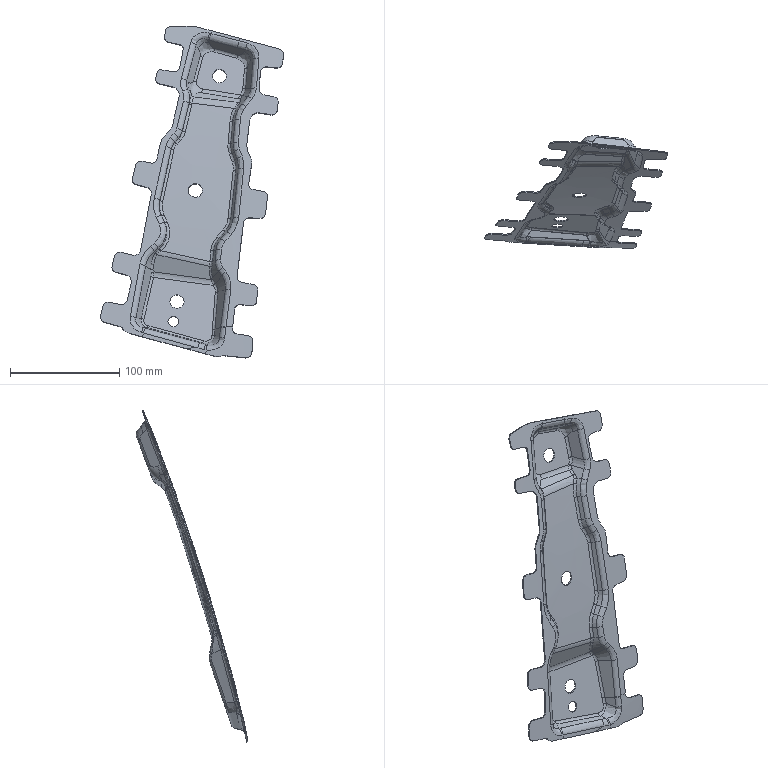Part | STEP file | FNA5401531 | 1 solid | 404 faces | box 167.899 x 102.592 x 304.372 mm | volume 32215 mm3 | spline 356 | cylinder 26 | plane 18 | other 4 | commonest cylinder face diameters 6 x5 8 x5 13 x4 10 x2 20 x2 22 x2